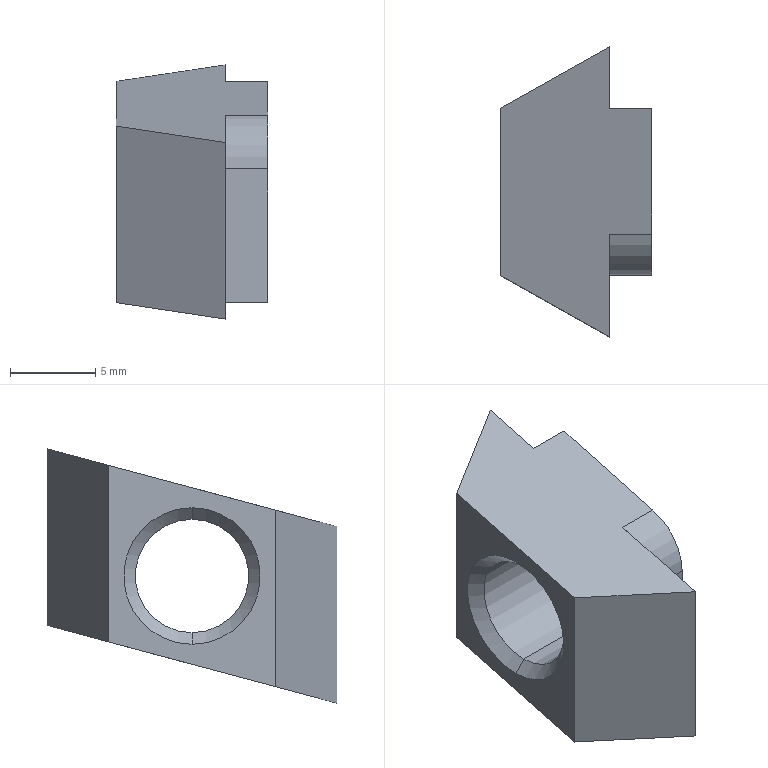Part | STEP file | 0245_014_HNTFSN8-8 | 1 solid | 18 faces | box 8.9 x 17 x 14.908 mm | volume 816.432 mm3 | plane 10 | cone 4 | cylinder 4 | commonest cylinder face diameters 6.533 x2 6.647 x2
STEP:
#1=CARTESIAN_POINT('',(0.,0.,0.));
#2=DIRECTION('',(0.,0.,1.));
#3=DIRECTION('',(1.,0.,0.));
#4=AXIS2_PLACEMENT_3D('',#1,#2,#3);
#5=CARTESIAN_POINT('',(-8.223,0.,3.323));
#6=VERTEX_POINT('',#5);
#7=CARTESIAN_POINT('',(-8.9,0.,4.));
#8=VERTEX_POINT('',#7);
#9=CARTESIAN_POINT('',(-8.9,0.,4.));
#10=DIRECTION('',(-0.7071,0.,0.7071));
#11=VECTOR('',#10,1.);
#12=LINE('',#9,#11);
#13=CARTESIAN_POINT('',(-8.9,0.,0.));
#14=DIRECTION('',(-1.,0.,0.));
#15=DIRECTION('',(0.,0.,1.));
#16=AXIS2_PLACEMENT_3D('',#13,#14,#15);
#17=CONICAL_SURFACE('',#16,4.,0.7854);
#18=CARTESIAN_POINT('',(6.283,0.));
#19=DIRECTION('',(0.,1.));
#20=VECTOR('',#19,1.);
#21=LINE('',#18,#20);
#22=(GEOMETRIC_REPRESENTATION_CONTEXT(2)PARAMETRIC_REPRESENTATION_CONTEXT()REPRESENTATION_CONTEXT('',''));
#23=DEFINITIONAL_REPRESENTATION('',(#21),#22);
#24=PCURVE('',#17,#23);
#25=CARTESIAN_POINT('',(-8.9,0.,0.));
#26=DIRECTION('',(-1.,0.,0.));
#27=DIRECTION('',(0.,0.,1.));
#28=AXIS2_PLACEMENT_3D('',#25,#26,#27);
#29=CONICAL_SURFACE('',#28,4.,0.7854);
#30=CARTESIAN_POINT('',(0.,0.));
#31=DIRECTION('',(0.,1.));
#32=VECTOR('',#31,1.);
#33=LINE('',#30,#32);
#34=(GEOMETRIC_REPRESENTATION_CONTEXT(2)PARAMETRIC_REPRESENTATION_CONTEXT()REPRESENTATION_CONTEXT('',''));
#35=DEFINITIONAL_REPRESENTATION('',(#33),#34);
#36=PCURVE('',#29,#35);
#37=SURFACE_CURVE('',#12,(#24,#36),.PCURVE_S1.);
#38=EDGE_CURVE('',#6,#8,#37,.T.);
#39=ORIENTED_EDGE('',*,*,#38,.T.);
#40=CARTESIAN_POINT('',(-8.9,0.,-4.));
#41=VERTEX_POINT('',#40);
#42=CARTESIAN_POINT('',(-8.9,0.,0.));
#43=DIRECTION('',(-1.,0.,0.));
#44=DIRECTION('',(0.,0.,1.));
#45=AXIS2_PLACEMENT_3D('',#42,#43,#44);
#46=CIRCLE('',#45,4.);
#47=CARTESIAN_POINT('',(0.,0.));
#48=DIRECTION('',(1.,0.));
#49=VECTOR('',#48,1.);
#50=LINE('',#47,#49);
#51=(GEOMETRIC_REPRESENTATION_CONTEXT(2)PARAMETRIC_REPRESENTATION_CONTEXT()REPRESENTATION_CONTEXT('',''));
#52=DEFINITIONAL_REPRESENTATION('',(#50),#51);
#53=PCURVE('',#17,#52);
#54=CARTESIAN_POINT('',(-8.9,0.,0.));
#55=DIRECTION('',(1.,0.,0.));
#56=DIRECTION('',(0.,0.,-1.));
#57=AXIS2_PLACEMENT_3D('',#54,#55,#56);
#58=PLANE('',#57);
#59=CARTESIAN_POINT('',(-4.,0.));
#60=CARTESIAN_POINT('',(-4.,6.928));
#61=CARTESIAN_POINT('',(2.,3.464));
#62=CARTESIAN_POINT('',(8.,0.));
#63=CARTESIAN_POINT('',(2.,-3.464));
#64=CARTESIAN_POINT('',(-4.,-6.928));
#65=CARTESIAN_POINT('',(-4.,0.));
#66=(BOUNDED_CURVE()B_SPLINE_CURVE(2,(#59,#60,#61,#62,#63,#64,#65),.UNSPECIFIED.,.T.,.F.)B_SPLINE_CURVE_WITH_KNOTS((1,2,2,2,2,1),(-2.094,0.,2.094,4.189,6.283,8.378),.UNSPECIFIED.)CURVE()GEOMETRIC_REPRESENTATION_ITEM()RATIONAL_B_SPLINE_CURVE((1.,0.5,1.,0.5,1.,0.5,1.))REPRESENTATION_ITEM(''));
#67=(GEOMETRIC_REPRESENTATION_CONTEXT(2)PARAMETRIC_REPRESENTATION_CONTEXT()REPRESENTATION_CONTEXT('',''));
#68=DEFINITIONAL_REPRESENTATION('',(#66),#67);
#69=PCURVE('',#58,#68);
#70=SURFACE_CURVE('',#46,(#53,#69),.PCURVE_S1.);
#71=EDGE_CURVE('',#41,#8,#70,.T.);
#72=ORIENTED_EDGE('',*,*,#71,.F.);
#73=CARTESIAN_POINT('',(-8.223,0.,-3.323));
#74=VERTEX_POINT('',#73);
#75=CARTESIAN_POINT('',(-8.9,0.,-4.));
#76=DIRECTION('',(-0.7071,0.,-0.7071));
#77=VECTOR('',#76,1.);
#78=LINE('',#75,#77);
#79=CARTESIAN_POINT('',(3.142,0.));
#80=DIRECTION('',(0.,1.));
#81=VECTOR('',#80,1.);
#82=LINE('',#79,#81);
#83=(GEOMETRIC_REPRESENTATION_CONTEXT(2)PARAMETRIC_REPRESENTATION_CONTEXT()REPRESENTATION_CONTEXT('',''));
#84=DEFINITIONAL_REPRESENTATION('',(#82),#83);
#85=PCURVE('',#17,#84);
#86=CARTESIAN_POINT('',(3.142,0.));
#87=DIRECTION('',(0.,1.));
#88=VECTOR('',#87,1.);
#89=LINE('',#86,#88);
#90=(GEOMETRIC_REPRESENTATION_CONTEXT(2)PARAMETRIC_REPRESENTATION_CONTEXT()REPRESENTATION_CONTEXT('',''));
#91=DEFINITIONAL_REPRESENTATION('',(#89),#90);
#92=PCURVE('',#29,#91);
#93=SURFACE_CURVE('',#78,(#85,#92),.PCURVE_S1.);
#94=EDGE_CURVE('',#74,#41,#93,.T.);
#95=ORIENTED_EDGE('',*,*,#94,.F.);
#96=CARTESIAN_POINT('',(-8.223,0.,0.));
#97=DIRECTION('',(-1.,0.,0.));
#98=DIRECTION('',(0.,1.,0.));
#99=AXIS2_PLACEMENT_3D('',#96,#97,#98);
#100=CIRCLE('',#99,3.323);
#101=CARTESIAN_POINT('',(1.571,-0.6765));
#102=DIRECTION('',(1.,0.));
#103=VECTOR('',#102,1.);
#104=LINE('',#101,#103);
#105=(GEOMETRIC_REPRESENTATION_CONTEXT(2)PARAMETRIC_REPRESENTATION_CONTEXT()REPRESENTATION_CONTEXT('',''));
#106=DEFINITIONAL_REPRESENTATION('',(#104),#105);
#107=PCURVE('',#17,#106);
#108=CARTESIAN_POINT('',(-4.45,0.,0.));
#109=DIRECTION('',(1.,0.,0.));
#110=DIRECTION('',(0.,0.,-1.));
#111=AXIS2_PLACEMENT_3D('',#108,#109,#110);
#112=CYLINDRICAL_SURFACE('',#111,3.324);
#113=CARTESIAN_POINT('',(7.854,-3.773));
#114=DIRECTION('',(-1.,0.));
#115=VECTOR('',#114,1.);
#116=LINE('',#113,#115);
#117=(GEOMETRIC_REPRESENTATION_CONTEXT(2)PARAMETRIC_REPRESENTATION_CONTEXT()REPRESENTATION_CONTEXT('',''));
#118=DEFINITIONAL_REPRESENTATION('',(#116),#117);
#119=PCURVE('',#112,#118);
#120=SURFACE_CURVE('',#100,(#107,#119),.PCURVE_S1.);
#121=EDGE_CURVE('',#74,#6,#120,.T.);
#122=ORIENTED_EDGE('',*,*,#121,.T.);
#123=EDGE_LOOP('',(#39,#72,#95,#122));
#124=FACE_BOUND('',#123,.F.);
#125=ADVANCED_FACE('',(#124),#17,.F.);
#126=CARTESIAN_POINT('',(-0.6765,0.,-3.324));
#127=VERTEX_POINT('',#126);
#128=CARTESIAN_POINT('',(0.,0.,-4.));
#129=VERTEX_POINT('',#128);
#130=CARTESIAN_POINT('',(0.,0.,-4.));
#131=DIRECTION('',(0.7071,0.,-0.7071));
#132=VECTOR('',#131,1.);
#133=LINE('',#130,#132);
#134=CARTESIAN_POINT('',(0.,0.,0.));
#135=DIRECTION('',(1.,0.,0.));
#136=DIRECTION('',(0.,0.,-1.));
#137=AXIS2_PLACEMENT_3D('',#134,#135,#136);
#138=CONICAL_SURFACE('',#137,4.,0.7854);
#139=CARTESIAN_POINT('',(6.283,0.));
#140=DIRECTION('',(0.,1.));
#141=VECTOR('',#140,1.);
#142=LINE('',#139,#141);
#143=(GEOMETRIC_REPRESENTATION_CONTEXT(2)PARAMETRIC_REPRESENTATION_CONTEXT()REPRESENTATION_CONTEXT('',''));
#144=DEFINITIONAL_REPRESENTATION('',(#142),#143);
#145=PCURVE('',#138,#144);
#146=CARTESIAN_POINT('',(0.,0.,0.));
#147=DIRECTION('',(1.,0.,0.));
#148=DIRECTION('',(0.,0.,-1.));
#149=AXIS2_PLACEMENT_3D('',#146,#147,#148);
#150=CONICAL_SURFACE('',#149,4.,0.7854);
#151=CARTESIAN_POINT('',(0.,0.));
#152=DIRECTION('',(0.,1.));
#153=VECTOR('',#152,1.);
#154=LINE('',#151,#153);
#155=(GEOMETRIC_REPRESENTATION_CONTEXT(2)PARAMETRIC_REPRESENTATION_CONTEXT()REPRESENTATION_CONTEXT('',''));
#156=DEFINITIONAL_REPRESENTATION('',(#154),#155);
#157=PCURVE('',#150,#156);
#158=SURFACE_CURVE('',#133,(#145,#157),.PCURVE_S1.);
#159=EDGE_CURVE('',#127,#129,#158,.T.);
#160=ORIENTED_EDGE('',*,*,#159,.T.);
#161=CARTESIAN_POINT('',(0.,0.,4.));
#162=VERTEX_POINT('',#161);
#163=CARTESIAN_POINT('',(0.,0.,0.));
#164=DIRECTION('',(-1.,0.,0.));
#165=DIRECTION('',(0.,0.,-1.));
#166=AXIS2_PLACEMENT_3D('',#163,#164,#165);
#167=CIRCLE('',#166,4.);
#168=CARTESIAN_POINT('',(6.283,0.));
#169=DIRECTION('',(-1.,0.));
#170=VECTOR('',#169,1.);
#171=LINE('',#168,#170);
#172=(GEOMETRIC_REPRESENTATION_CONTEXT(2)PARAMETRIC_REPRESENTATION_CONTEXT()REPRESENTATION_CONTEXT('',''));
#173=DEFINITIONAL_REPRESENTATION('',(#171),#172);
#174=PCURVE('',#138,#173);
#175=CARTESIAN_POINT('',(0.,0.,0.));
#176=DIRECTION('',(1.,0.,0.));
#177=DIRECTION('',(0.,0.,-1.));
#178=AXIS2_PLACEMENT_3D('',#175,#176,#177);
#179=PLANE('',#178);
#180=CARTESIAN_POINT('',(4.,0.));
#181=CARTESIAN_POINT('',(4.,-6.928));
#182=CARTESIAN_POINT('',(-2.,-3.464));
#183=CARTESIAN_POINT('',(-8.,0.));
#184=CARTESIAN_POINT('',(-2.,3.464));
#185=CARTESIAN_POINT('',(4.,6.928));
#186=CARTESIAN_POINT('',(4.,0.));
#187=(BOUNDED_CURVE()B_SPLINE_CURVE(2,(#180,#181,#182,#183,#184,#185,#186),.UNSPECIFIED.,.T.,.F.)B_SPLINE_CURVE_WITH_KNOTS((1,2,2,2,2,1),(-2.094,0.,2.094,4.189,6.283,8.378),.UNSPECIFIED.)CURVE()GEOMETRIC_REPRESENTATION_ITEM()RATIONAL_B_SPLINE_CURVE((1.,0.5,1.,0.5,1.,0.5,1.))REPRESENTATION_ITEM(''));
#188=(GEOMETRIC_REPRESENTATION_CONTEXT(2)PARAMETRIC_REPRESENTATION_CONTEXT()REPRESENTATION_CONTEXT('',''));
#189=DEFINITIONAL_REPRESENTATION('',(#187),#188);
#190=PCURVE('',#179,#189);
#191=SURFACE_CURVE('',#167,(#174,#190),.PCURVE_S1.);
#192=EDGE_CURVE('',#129,#162,#191,.T.);
#193=ORIENTED_EDGE('',*,*,#192,.T.);
#194=CARTESIAN_POINT('',(-0.6765,0.,3.324));
#195=VERTEX_POINT('',#194);
#196=CARTESIAN_POINT('',(0.,0.,4.));
#197=DIRECTION('',(0.7071,0.,0.7071));
#198=VECTOR('',#197,1.);
#199=LINE('',#196,#198);
#200=CARTESIAN_POINT('',(3.142,0.));
#201=DIRECTION('',(0.,1.));
#202=VECTOR('',#201,1.);
#203=LINE('',#200,#202);
#204=(GEOMETRIC_REPRESENTATION_CONTEXT(2)PARAMETRIC_REPRESENTATION_CONTEXT()REPRESENTATION_CONTEXT('',''));
#205=DEFINITIONAL_REPRESENTATION('',(#203),#204);
#206=PCURVE('',#138,#205);
#207=CARTESIAN_POINT('',(3.142,0.));
#208=DIRECTION('',(0.,1.));
#209=VECTOR('',#208,1.);
#210=LINE('',#207,#209);
#211=(GEOMETRIC_REPRESENTATION_CONTEXT(2)PARAMETRIC_REPRESENTATION_CONTEXT()REPRESENTATION_CONTEXT('',''));
#212=DEFINITIONAL_REPRESENTATION('',(#210),#211);
#213=PCURVE('',#150,#212);
#214=SURFACE_CURVE('',#199,(#206,#213),.PCURVE_S1.);
#215=EDGE_CURVE('',#195,#162,#214,.T.);
#216=ORIENTED_EDGE('',*,*,#215,.F.);
#217=CARTESIAN_POINT('',(-0.6765,0.,0.));
#218=DIRECTION('',(1.,0.,0.));
#219=DIRECTION('',(0.,1.,0.));
#220=AXIS2_PLACEMENT_3D('',#217,#218,#219);
#221=CIRCLE('',#220,3.324);
#222=CARTESIAN_POINT('',(1.571,-0.6765));
#223=DIRECTION('',(1.,0.));
#224=VECTOR('',#223,1.);
#225=LINE('',#222,#224);
#226=(GEOMETRIC_REPRESENTATION_CONTEXT(2)PARAMETRIC_REPRESENTATION_CONTEXT()REPRESENTATION_CONTEXT('',''));
#227=DEFINITIONAL_REPRESENTATION('',(#225),#226);
#228=PCURVE('',#138,#227);
#229=CARTESIAN_POINT('',(1.571,3.774));
#230=DIRECTION('',(1.,0.));
#231=VECTOR('',#230,1.);
#232=LINE('',#229,#231);
#233=(GEOMETRIC_REPRESENTATION_CONTEXT(2)PARAMETRIC_REPRESENTATION_CONTEXT()REPRESENTATION_CONTEXT('',''));
#234=DEFINITIONAL_REPRESENTATION('',(#232),#233);
#235=PCURVE('',#112,#234);
#236=SURFACE_CURVE('',#221,(#228,#235),.PCURVE_S1.);
#237=EDGE_CURVE('',#195,#127,#236,.T.);
#238=ORIENTED_EDGE('',*,*,#237,.T.);
#239=EDGE_LOOP('',(#160,#193,#216,#238));
#240=FACE_BOUND('',#239,.F.);
#241=ADVANCED_FACE('',(#240),#138,.F.);
#242=CARTESIAN_POINT('',(-4.45,0.,-3.324));
#243=DIRECTION('',(1.,0.,0.));
#244=VECTOR('',#243,1.);
#245=LINE('',#242,#244);
#246=CARTESIAN_POINT('',(6.283,0.));
#247=DIRECTION('',(0.,1.));
#248=VECTOR('',#247,1.);
#249=LINE('',#246,#248);
#250=(GEOMETRIC_REPRESENTATION_CONTEXT(2)PARAMETRIC_REPRESENTATION_CONTEXT()REPRESENTATION_CONTEXT('',''));
#251=DEFINITIONAL_REPRESENTATION('',(#249),#250);
#252=PCURVE('',#112,#251);
#253=CARTESIAN_POINT('',(-4.45,0.,0.));
#254=DIRECTION('',(1.,0.,0.));
#255=DIRECTION('',(0.,0.,-1.));
#256=AXIS2_PLACEMENT_3D('',#253,#254,#255);
#257=CYLINDRICAL_SURFACE('',#256,3.324);
#258=CARTESIAN_POINT('',(0.,0.));
#259=DIRECTION('',(0.,1.));
#260=VECTOR('',#259,1.);
#261=LINE('',#258,#260);
#262=(GEOMETRIC_REPRESENTATION_CONTEXT(2)PARAMETRIC_REPRESENTATION_CONTEXT()REPRESENTATION_CONTEXT('',''));
#263=DEFINITIONAL_REPRESENTATION('',(#261),#262);
#264=PCURVE('',#257,#263);
#265=SURFACE_CURVE('',#245,(#252,#264),.PCURVE_S1.);
#266=EDGE_CURVE('',#74,#127,#265,.T.);
#267=ORIENTED_EDGE('',*,*,#266,.T.);
#268=ORIENTED_EDGE('',*,*,#237,.F.);
#269=CARTESIAN_POINT('',(-4.45,0.,3.324));
#270=DIRECTION('',(1.,0.,0.));
#271=VECTOR('',#270,1.);
#272=LINE('',#269,#271);
#273=CARTESIAN_POINT('',(3.142,0.));
#274=DIRECTION('',(0.,1.));
#275=VECTOR('',#274,1.);
#276=LINE('',#273,#275);
#277=(GEOMETRIC_REPRESENTATION_CONTEXT(2)PARAMETRIC_REPRESENTATION_CONTEXT()REPRESENTATION_CONTEXT('',''));
#278=DEFINITIONAL_REPRESENTATION('',(#276),#277);
#279=PCURVE('',#112,#278);
#280=CARTESIAN_POINT('',(3.142,0.));
#281=DIRECTION('',(0.,1.));
#282=VECTOR('',#281,1.);
#283=LINE('',#280,#282);
#284=(GEOMETRIC_REPRESENTATION_CONTEXT(2)PARAMETRIC_REPRESENTATION_CONTEXT()REPRESENTATION_CONTEXT('',''));
#285=DEFINITIONAL_REPRESENTATION('',(#283),#284);
#286=PCURVE('',#257,#285);
#287=SURFACE_CURVE('',#272,(#279,#286),.PCURVE_S1.);
#288=EDGE_CURVE('',#6,#195,#287,.T.);
#289=ORIENTED_EDGE('',*,*,#288,.F.);
#290=ORIENTED_EDGE('',*,*,#121,.F.);
#291=EDGE_LOOP('',(#267,#268,#289,#290));
#292=FACE_BOUND('',#291,.F.);
#293=ADVANCED_FACE('',(#292),#112,.F.);
#294=CARTESIAN_POINT('',(-8.9,-4.9,3.863));
#295=VERTEX_POINT('',#294);
#296=CARTESIAN_POINT('',(-2.5,-8.5,2.899));
#297=VERTEX_POINT('',#296);
#298=CARTESIAN_POINT('',(-8.9,-4.9,3.863));
#299=DIRECTION('',(0.8642,-0.4861,-0.1302));
#300=VECTOR('',#299,1.);
#301=LINE('',#298,#300);
#302=CARTESIAN_POINT('',(0.,8.5,7.454));
#303=DIRECTION('',(0.,-0.2588,0.9659));
#304=DIRECTION('',(0.,-0.9659,-0.2588));
#305=AXIS2_PLACEMENT_3D('',#302,#303,#304);
#306=PLANE('',#305);
#307=CARTESIAN_POINT('',(13.873,-8.9));
#308=DIRECTION('',(0.5032,0.8642));
#309=VECTOR('',#308,1.);
#310=LINE('',#307,#309);
#311=(GEOMETRIC_REPRESENTATION_CONTEXT(2)PARAMETRIC_REPRESENTATION_CONTEXT()REPRESENTATION_CONTEXT('',''));
#312=DEFINITIONAL_REPRESENTATION('',(#310),#311);
#313=PCURVE('',#306,#312);
#314=CARTESIAN_POINT('',(-2.5,-8.5,20.));
#315=DIRECTION('',(0.4903,0.8716,0.));
#316=DIRECTION('',(-0.8716,0.4903,0.));
#317=AXIS2_PLACEMENT_3D('',#314,#315,#316);
#318=PLANE('',#317);
#319=CARTESIAN_POINT('',(7.343,-16.137));
#320=DIRECTION('',(-0.9915,-0.1302));
#321=VECTOR('',#320,1.);
#322=LINE('',#319,#321);
#323=(GEOMETRIC_REPRESENTATION_CONTEXT(2)PARAMETRIC_REPRESENTATION_CONTEXT()REPRESENTATION_CONTEXT('',''));
#324=DEFINITIONAL_REPRESENTATION('',(#322),#323);
#325=PCURVE('',#318,#324);
#326=SURFACE_CURVE('',#301,(#313,#325),.PCURVE_S1.);
#327=EDGE_CURVE('',#295,#297,#326,.T.);
#328=ORIENTED_EDGE('',*,*,#327,.T.);
#329=CARTESIAN_POINT('',(-2.5,-2.479,4.512));
#330=VERTEX_POINT('',#329);
#331=CARTESIAN_POINT('',(-2.5,8.5,7.454));
#332=DIRECTION('',(0.,0.9659,0.2588));
#333=VECTOR('',#332,1.);
#334=LINE('',#331,#333);
#335=CARTESIAN_POINT('',(0.,-2.5));
#336=DIRECTION('',(-1.,0.));
#337=VECTOR('',#336,1.);
#338=LINE('',#335,#337);
#339=(GEOMETRIC_REPRESENTATION_CONTEXT(2)PARAMETRIC_REPRESENTATION_CONTEXT()REPRESENTATION_CONTEXT('',''));
#340=DEFINITIONAL_REPRESENTATION('',(#338),#339);
#341=PCURVE('',#306,#340);
#342=CARTESIAN_POINT('',(-2.5,-4.9,20.));
#343=DIRECTION('',(-1.,0.,0.));
#344=DIRECTION('',(0.,0.,1.));
#345=AXIS2_PLACEMENT_3D('',#342,#343,#344);
#346=PLANE('',#345);
#347=CARTESIAN_POINT('',(-12.546,13.4));
#348=DIRECTION('',(0.2588,0.9659));
#349=VECTOR('',#348,1.);
#350=LINE('',#347,#349);
#351=(GEOMETRIC_REPRESENTATION_CONTEXT(2)PARAMETRIC_REPRESENTATION_CONTEXT()REPRESENTATION_CONTEXT('',''));
#352=DEFINITIONAL_REPRESENTATION('',(#350),#351);
#353=PCURVE('',#346,#352);
#354=SURFACE_CURVE('',#334,(#341,#353),.PCURVE_S1.);
#355=EDGE_CURVE('',#297,#330,#354,.T.);
#356=ORIENTED_EDGE('',*,*,#355,.T.);
#357=CARTESIAN_POINT('',(0.,-2.479,4.512));
#358=VERTEX_POINT('',#357);
#359=CARTESIAN_POINT('',(0.,-2.479,4.512));
#360=DIRECTION('',(1.,0.,0.));
#361=VECTOR('',#360,1.);
#362=LINE('',#359,#361);
#363=CARTESIAN_POINT('',(11.366,0.));
#364=DIRECTION('',(0.,1.));
#365=VECTOR('',#364,1.);
#366=LINE('',#363,#365);
#367=(GEOMETRIC_REPRESENTATION_CONTEXT(2)PARAMETRIC_REPRESENTATION_CONTEXT()REPRESENTATION_CONTEXT('',''));
#368=DEFINITIONAL_REPRESENTATION('',(#366),#367);
#369=PCURVE('',#306,#368);
#370=CARTESIAN_POINT('',(-2.5,-1.633,1.357));
#371=DIRECTION('',(-1.,0.,0.));
#372=DIRECTION('',(0.,0.,1.));
#373=AXIS2_PLACEMENT_3D('',#370,#371,#372);
#374=CYLINDRICAL_SURFACE('',#373,3.267);
#375=CARTESIAN_POINT('',(6.021,-2.5));
#376=DIRECTION('',(0.,-1.));
#377=VECTOR('',#376,1.);
#378=LINE('',#375,#377);
#379=(GEOMETRIC_REPRESENTATION_CONTEXT(2)PARAMETRIC_REPRESENTATION_CONTEXT()REPRESENTATION_CONTEXT('',''));
#380=DEFINITIONAL_REPRESENTATION('',(#378),#379);
#381=PCURVE('',#374,#380);
#382=SURFACE_CURVE('',#362,(#369,#381),.PCURVE_S1.);
#383=EDGE_CURVE('',#330,#358,#382,.T.);
#384=ORIENTED_EDGE('',*,*,#383,.T.);
#385=CARTESIAN_POINT('',(0.,4.9,6.489));
#386=VERTEX_POINT('',#385);
#387=CARTESIAN_POINT('',(0.,8.5,7.454));
#388=DIRECTION('',(0.,0.9659,0.2588));
#389=VECTOR('',#388,1.);
#390=LINE('',#387,#389);
#391=CARTESIAN_POINT('',(0.,0.));
#392=DIRECTION('',(-1.,0.));
#393=VECTOR('',#392,1.);
#394=LINE('',#391,#393);
#395=(GEOMETRIC_REPRESENTATION_CONTEXT(2)PARAMETRIC_REPRESENTATION_CONTEXT()REPRESENTATION_CONTEXT('',''));
#396=DEFINITIONAL_REPRESENTATION('',(#394),#395);
#397=PCURVE('',#306,#396);
#398=CARTESIAN_POINT('',(-7.454,8.5));
#399=DIRECTION('',(-0.2588,0.9659));
#400=VECTOR('',#399,1.);
#401=LINE('',#398,#400);
#402=(GEOMETRIC_REPRESENTATION_CONTEXT(2)PARAMETRIC_REPRESENTATION_CONTEXT()REPRESENTATION_CONTEXT('',''));
#403=DEFINITIONAL_REPRESENTATION('',(#401),#402);
#404=PCURVE('',#179,#403);
#405=SURFACE_CURVE('',#390,(#397,#404),.PCURVE_S1.);
#406=EDGE_CURVE('',#358,#386,#405,.T.);
#407=ORIENTED_EDGE('',*,*,#406,.T.);
#408=CARTESIAN_POINT('',(-2.5,4.9,6.489));
#409=VERTEX_POINT('',#408);
#410=CARTESIAN_POINT('',(0.,4.9,6.489));
#411=DIRECTION('',(-1.,0.,0.));
#412=VECTOR('',#411,1.);
#413=LINE('',#410,#412);
#414=CARTESIAN_POINT('',(3.727,0.));
#415=DIRECTION('',(0.,-1.));
#416=VECTOR('',#415,1.);
#417=LINE('',#414,#416);
#418=(GEOMETRIC_REPRESENTATION_CONTEXT(2)PARAMETRIC_REPRESENTATION_CONTEXT()REPRESENTATION_CONTEXT('',''));
#419=DEFINITIONAL_REPRESENTATION('',(#417),#418);
#420=PCURVE('',#306,#419);
#421=CARTESIAN_POINT('',(-2.5,4.9,20.));
#422=DIRECTION('',(0.,-1.,0.));
#423=DIRECTION('',(1.,0.,0.));
#424=AXIS2_PLACEMENT_3D('',#421,#422,#423);
#425=PLANE('',#424);
#426=CARTESIAN_POINT('',(2.5,-13.511));
#427=DIRECTION('',(-1.,0.));
#428=VECTOR('',#427,1.);
#429=LINE('',#426,#428);
#430=(GEOMETRIC_REPRESENTATION_CONTEXT(2)PARAMETRIC_REPRESENTATION_CONTEXT()REPRESENTATION_CONTEXT('',''));
#431=DEFINITIONAL_REPRESENTATION('',(#429),#430);
#432=PCURVE('',#425,#431);
#433=SURFACE_CURVE('',#413,(#420,#432),.PCURVE_S1.);
#434=EDGE_CURVE('',#386,#409,#433,.T.);
#435=ORIENTED_EDGE('',*,*,#434,.T.);
#436=CARTESIAN_POINT('',(-2.5,8.5,7.454));
#437=VERTEX_POINT('',#436);
#438=CARTESIAN_POINT('',(-2.5,8.5,7.454));
#439=DIRECTION('',(0.,0.9659,0.2588));
#440=VECTOR('',#439,1.);
#441=LINE('',#438,#440);
#442=CARTESIAN_POINT('',(0.,-2.5));
#443=DIRECTION('',(-1.,0.));
#444=VECTOR('',#443,1.);
#445=LINE('',#442,#444);
#446=(GEOMETRIC_REPRESENTATION_CONTEXT(2)PARAMETRIC_REPRESENTATION_CONTEXT()REPRESENTATION_CONTEXT('',''));
#447=DEFINITIONAL_REPRESENTATION('',(#445),#446);
#448=PCURVE('',#306,#447);
#449=CARTESIAN_POINT('',(-2.5,8.5,20.));
#450=DIRECTION('',(-1.,0.,0.));
#451=DIRECTION('',(0.,0.,1.));
#452=AXIS2_PLACEMENT_3D('',#449,#450,#451);
#453=PLANE('',#452);
#454=CARTESIAN_POINT('',(-12.546,0.));
#455=DIRECTION('',(0.2588,0.9659));
#456=VECTOR('',#455,1.);
#457=LINE('',#454,#456);
#458=(GEOMETRIC_REPRESENTATION_CONTEXT(2)PARAMETRIC_REPRESENTATION_CONTEXT()REPRESENTATION_CONTEXT('',''));
#459=DEFINITIONAL_REPRESENTATION('',(#457),#458);
#460=PCURVE('',#453,#459);
#461=SURFACE_CURVE('',#441,(#448,#460),.PCURVE_S1.);
#462=EDGE_CURVE('',#409,#437,#461,.T.);
#463=ORIENTED_EDGE('',*,*,#462,.T.);
#464=CARTESIAN_POINT('',(-8.9,4.9,6.489));
#465=VERTEX_POINT('',#464);
#466=CARTESIAN_POINT('',(-2.5,8.5,7.454));
#467=DIRECTION('',(-0.8642,-0.4861,-0.1302));
#468=VECTOR('',#467,1.);
#469=LINE('',#466,#468);
#470=CARTESIAN_POINT('',(0.,-2.5));
#471=DIRECTION('',(0.5032,-0.8642));
#472=VECTOR('',#471,1.);
#473=LINE('',#470,#472);
#474=(GEOMETRIC_REPRESENTATION_CONTEXT(2)PARAMETRIC_REPRESENTATION_CONTEXT()REPRESENTATION_CONTEXT('',''));
#475=DEFINITIONAL_REPRESENTATION('',(#473),#474);
#476=PCURVE('',#306,#475);
#477=CARTESIAN_POINT('',(-8.9,4.9,20.));
#478=DIRECTION('',(0.4903,-0.8716,0.));
#479=DIRECTION('',(0.8716,0.4903,0.));
#480=AXIS2_PLACEMENT_3D('',#477,#478,#479);
#481=PLANE('',#480);
#482=CARTESIAN_POINT('',(7.343,-12.546));
#483=DIRECTION('',(-0.9915,-0.1302));
#484=VECTOR('',#483,1.);
#485=LINE('',#482,#484);
#486=(GEOMETRIC_REPRESENTATION_CONTEXT(2)PARAMETRIC_REPRESENTATION_CONTEXT()REPRESENTATION_CONTEXT('',''));
#487=DEFINITIONAL_REPRESENTATION('',(#485),#486);
#488=PCURVE('',#481,#487);
#489=SURFACE_CURVE('',#469,(#476,#488),.PCURVE_S1.);
#490=EDGE_CURVE('',#437,#465,#489,.T.);
#491=ORIENTED_EDGE('',*,*,#490,.T.);
#492=CARTESIAN_POINT('',(-8.9,8.5,7.454));
#493=DIRECTION('',(0.,-0.9659,-0.2588));
#494=VECTOR('',#493,1.);
#495=LINE('',#492,#494);
#496=CARTESIAN_POINT('',(0.,-8.9));
#497=DIRECTION('',(1.,0.));
#498=VECTOR('',#497,1.);
#499=LINE('',#496,#498);
#500=(GEOMETRIC_REPRESENTATION_CONTEXT(2)PARAMETRIC_REPRESENTATION_CONTEXT()REPRESENTATION_CONTEXT('',''));
#501=DEFINITIONAL_REPRESENTATION('',(#499),#500);
#502=PCURVE('',#306,#501);
#503=CARTESIAN_POINT('',(-7.454,8.5));
#504=DIRECTION('',(0.2588,-0.9659));
#505=VECTOR('',#504,1.);
#506=LINE('',#503,#505);
#507=(GEOMETRIC_REPRESENTATION_CONTEXT(2)PARAMETRIC_REPRESENTATION_CONTEXT()REPRESENTATION_CONTEXT('',''));
#508=DEFINITIONAL_REPRESENTATION('',(#506),#507);
#509=PCURVE('',#58,#508);
#510=SURFACE_CURVE('',#495,(#502,#509),.PCURVE_S1.);
#511=EDGE_CURVE('',#465,#295,#510,.T.);
#512=ORIENTED_EDGE('',*,*,#511,.T.);
#513=EDGE_LOOP('',(#328,#356,#384,#407,#435,#463,#491,#512));
#514=FACE_BOUND('',#513,.T.);
#515=ADVANCED_FACE('',(#514),#306,.T.);
#516=CARTESIAN_POINT('',(-2.5,-8.5,-7.454));
#517=VERTEX_POINT('',#516);
#518=CARTESIAN_POINT('',(-2.5,-8.5,20.));
#519=DIRECTION('',(0.,0.,1.));
#520=VECTOR('',#519,1.);
#521=LINE('',#518,#520);
#522=CARTESIAN_POINT('',(0.,-3.6));
#523=DIRECTION('',(1.,0.));
#524=VECTOR('',#523,1.);
#525=LINE('',#522,#524);
#526=(GEOMETRIC_REPRESENTATION_CONTEXT(2)PARAMETRIC_REPRESENTATION_CONTEXT()REPRESENTATION_CONTEXT('',''));
#527=DEFINITIONAL_REPRESENTATION('',(#525),#526);
#528=PCURVE('',#346,#527);
#529=CARTESIAN_POINT('',(0.,0.));
#530=DIRECTION('',(0.,1.));
#531=VECTOR('',#530,1.);
#532=LINE('',#529,#531);
#533=(GEOMETRIC_REPRESENTATION_CONTEXT(2)PARAMETRIC_REPRESENTATION_CONTEXT()REPRESENTATION_CONTEXT('',''));
#534=DEFINITIONAL_REPRESENTATION('',(#532),#533);
#535=PCURVE('',#318,#534);
#536=SURFACE_CURVE('',#521,(#528,#535),.PCURVE_S1.);
#537=EDGE_CURVE('',#517,#297,#536,.T.);
#538=ORIENTED_EDGE('',*,*,#537,.F.);
#539=CARTESIAN_POINT('',(-2.5,-4.9,-6.489));
#540=VERTEX_POINT('',#539);
#541=CARTESIAN_POINT('',(-2.5,-4.9,-6.489));
#542=DIRECTION('',(0.,-0.9659,-0.2588));
#543=VECTOR('',#542,1.);
#544=LINE('',#541,#543);
#545=CARTESIAN_POINT('',(-26.489,0.));
#546=DIRECTION('',(-0.2588,-0.9659));
#547=VECTOR('',#546,1.);
#548=LINE('',#545,#547);
#549=(GEOMETRIC_REPRESENTATION_CONTEXT(2)PARAMETRIC_REPRESENTATION_CONTEXT()REPRESENTATION_CONTEXT('',''));
#550=DEFINITIONAL_REPRESENTATION('',(#548),#549);
#551=PCURVE('',#346,#550);
#552=CARTESIAN_POINT('',(0.,-8.5,-7.454));
#553=DIRECTION('',(0.,0.2588,-0.9659));
#554=DIRECTION('',(0.,0.9659,0.2588));
#555=AXIS2_PLACEMENT_3D('',#552,#553,#554);
#556=PLANE('',#555);
#557=CARTESIAN_POINT('',(3.727,-2.5));
#558=DIRECTION('',(-1.,0.));
#559=VECTOR('',#558,1.);
#560=LINE('',#557,#559);
#561=(GEOMETRIC_REPRESENTATION_CONTEXT(2)PARAMETRIC_REPRESENTATION_CONTEXT()REPRESENTATION_CONTEXT('',''));
#562=DEFINITIONAL_REPRESENTATION('',(#560),#561);
#563=PCURVE('',#556,#562);
#564=SURFACE_CURVE('',#544,(#551,#563),.PCURVE_S1.);
#565=EDGE_CURVE('',#540,#517,#564,.T.);
#566=ORIENTED_EDGE('',*,*,#565,.F.);
#567=CARTESIAN_POINT('',(-2.5,-4.9,1.357));
#568=VERTEX_POINT('',#567);
#569=CARTESIAN_POINT('',(-2.5,-4.9,20.));
#570=DIRECTION('',(0.,0.,-1.));
#571=VECTOR('',#570,1.);
#572=LINE('',#569,#571);
#573=CARTESIAN_POINT('',(0.,0.));
#574=DIRECTION('',(-1.,0.));
#575=VECTOR('',#574,1.);
#576=LINE('',#573,#575);
#577=(GEOMETRIC_REPRESENTATION_CONTEXT(2)PARAMETRIC_REPRESENTATION_CONTEXT()REPRESENTATION_CONTEXT('',''));
#578=DEFINITIONAL_REPRESENTATION('',(#576),#577);
#579=PCURVE('',#346,#578);
#580=CARTESIAN_POINT('',(0.,-4.9,20.));
#581=DIRECTION('',(0.,1.,0.));
#582=DIRECTION('',(-1.,0.,0.));
#583=AXIS2_PLACEMENT_3D('',#580,#581,#582);
#584=PLANE('',#583);
#585=CARTESIAN_POINT('',(2.5,0.));
#586=DIRECTION('',(0.,-1.));
#587=VECTOR('',#586,1.);
#588=LINE('',#585,#587);
#589=(GEOMETRIC_REPRESENTATION_CONTEXT(2)PARAMETRIC_REPRESENTATION_CONTEXT()REPRESENTATION_CONTEXT('',''));
#590=DEFINITIONAL_REPRESENTATION('',(#588),#589);
#591=PCURVE('',#584,#590);
#592=SURFACE_CURVE('',#572,(#579,#591),.PCURVE_S1.);
#593=EDGE_CURVE('',#568,#540,#592,.T.);
#594=ORIENTED_EDGE('',*,*,#593,.F.);
#595=CARTESIAN_POINT('',(-2.5,-1.633,1.357));
#596=DIRECTION('',(1.,0.,0.));
#597=DIRECTION('',(0.,0.,1.));
#598=AXIS2_PLACEMENT_3D('',#595,#596,#597);
#599=CIRCLE('',#598,3.267);
#600=CARTESIAN_POINT('',(-15.377,3.267));
#601=CARTESIAN_POINT('',(-15.377,-2.391));
#602=CARTESIAN_POINT('',(-20.277,0.4377));
#603=CARTESIAN_POINT('',(-25.177,3.267));
#604=CARTESIAN_POINT('',(-20.277,6.096));
#605=CARTESIAN_POINT('',(-15.377,8.925));
#606=CARTESIAN_POINT('',(-15.377,3.267));
#607=(BOUNDED_CURVE()B_SPLINE_CURVE(2,(#600,#601,#602,#603,#604,#605,#606),.UNSPECIFIED.,.T.,.F.)B_SPLINE_CURVE_WITH_KNOTS((1,2,2,2,2,1),(-2.094,0.,2.094,4.189,6.283,8.378),.UNSPECIFIED.)CURVE()GEOMETRIC_REPRESENTATION_ITEM()RATIONAL_B_SPLINE_CURVE((1.,0.5,1.,0.5,1.,0.5,1.))REPRESENTATION_ITEM(''));
#608=(GEOMETRIC_REPRESENTATION_CONTEXT(2)PARAMETRIC_REPRESENTATION_CONTEXT()REPRESENTATION_CONTEXT('',''));
#609=DEFINITIONAL_REPRESENTATION('',(#607),#608);
#610=PCURVE('',#346,#609);
#611=CARTESIAN_POINT('',(6.283,0.));
#612=DIRECTION('',(-1.,0.));
#613=VECTOR('',#612,1.);
#614=LINE('',#611,#613);
#615=(GEOMETRIC_REPRESENTATION_CONTEXT(2)PARAMETRIC_REPRESENTATION_CONTEXT()REPRESENTATION_CONTEXT('',''));
#616=DEFINITIONAL_REPRESENTATION('',(#614),#615);
#617=PCURVE('',#374,#616);
#618=SURFACE_CURVE('',#599,(#610,#617),.PCURVE_S1.);
#619=EDGE_CURVE('',#330,#568,#618,.T.);
#620=ORIENTED_EDGE('',*,*,#619,.F.);
#621=ORIENTED_EDGE('',*,*,#355,.F.);
#622=EDGE_LOOP('',(#538,#566,#594,#620,#621));
#623=FACE_BOUND('',#622,.T.);
#624=ADVANCED_FACE('',(#623),#346,.F.);
#625=ORIENTED_EDGE('',*,*,#537,.T.);
#626=ORIENTED_EDGE('',*,*,#327,.F.);
#627=CARTESIAN_POINT('',(-8.9,-4.9,-6.489));
#628=VERTEX_POINT('',#627);
#629=CARTESIAN_POINT('',(-8.9,-4.9,20.));
#630=DIRECTION('',(0.,0.,1.));
#631=VECTOR('',#630,1.);
#632=LINE('',#629,#631);
#633=CARTESIAN_POINT('',(7.343,0.));
#634=DIRECTION('',(0.,1.));
#635=VECTOR('',#634,1.);
#636=LINE('',#633,#635);
#637=(GEOMETRIC_REPRESENTATION_CONTEXT(2)PARAMETRIC_REPRESENTATION_CONTEXT()REPRESENTATION_CONTEXT('',''));
#638=DEFINITIONAL_REPRESENTATION('',(#636),#637);
#639=PCURVE('',#318,#638);
#640=CARTESIAN_POINT('',(-20.,-4.9));
#641=DIRECTION('',(-1.,0.));
#642=VECTOR('',#641,1.);
#643=LINE('',#640,#642);
#644=(GEOMETRIC_REPRESENTATION_CONTEXT(2)PARAMETRIC_REPRESENTATION_CONTEXT()REPRESENTATION_CONTEXT('',''));
#645=DEFINITIONAL_REPRESENTATION('',(#643),#644);
#646=PCURVE('',#58,#645);
#647=SURFACE_CURVE('',#632,(#639,#646),.PCURVE_S1.);
#648=EDGE_CURVE('',#628,#295,#647,.T.);
#649=ORIENTED_EDGE('',*,*,#648,.F.);
#650=CARTESIAN_POINT('',(-2.5,-8.5,-7.454));
#651=DIRECTION('',(-0.8642,0.4861,0.1302));
#652=VECTOR('',#651,1.);
#653=LINE('',#650,#652);
#654=CARTESIAN_POINT('',(0.,-27.454));
#655=DIRECTION('',(0.9915,0.1302));
#656=VECTOR('',#655,1.);
#657=LINE('',#654,#656);
#658=(GEOMETRIC_REPRESENTATION_CONTEXT(2)PARAMETRIC_REPRESENTATION_CONTEXT()REPRESENTATION_CONTEXT('',''));
#659=DEFINITIONAL_REPRESENTATION('',(#657),#658);
#660=PCURVE('',#318,#659);
#661=CARTESIAN_POINT('',(0.,-2.5));
#662=DIRECTION('',(0.5032,-0.8642));
#663=VECTOR('',#662,1.);
#664=LINE('',#661,#663);
#665=(GEOMETRIC_REPRESENTATION_CONTEXT(2)PARAMETRIC_REPRESENTATION_CONTEXT()REPRESENTATION_CONTEXT('',''));
#666=DEFINITIONAL_REPRESENTATION('',(#664),#665);
#667=PCURVE('',#556,#666);
#668=SURFACE_CURVE('',#653,(#660,#667),.PCURVE_S1.);
#669=EDGE_CURVE('',#517,#628,#668,.T.);
#670=ORIENTED_EDGE('',*,*,#669,.F.);
#671=EDGE_LOOP('',(#625,#626,#649,#670));
#672=FACE_BOUND('',#671,.T.);
#673=ADVANCED_FACE('',(#672),#318,.F.);
#674=CARTESIAN_POINT('',(-8.9,4.9,-3.863));
#675=VERTEX_POINT('',#674);
#676=CARTESIAN_POINT('',(-8.9,-4.9,-6.489));
#677=DIRECTION('',(0.,0.9659,0.2588));
#678=VECTOR('',#677,1.);
#679=LINE('',#676,#678);
#680=CARTESIAN_POINT('',(6.489,-4.9));
#681=DIRECTION('',(-0.2588,0.9659));
#682=VECTOR('',#681,1.);
#683=LINE('',#680,#682);
#684=(GEOMETRIC_REPRESENTATION_CONTEXT(2)PARAMETRIC_REPRESENTATION_CONTEXT()REPRESENTATION_CONTEXT('',''));
#685=DEFINITIONAL_REPRESENTATION('',(#683),#684);
#686=PCURVE('',#58,#685);
#687=CARTESIAN_POINT('',(3.727,-8.9));
#688=DIRECTION('',(1.,0.));
#689=VECTOR('',#688,1.);
#690=LINE('',#687,#689);
#691=(GEOMETRIC_REPRESENTATION_CONTEXT(2)PARAMETRIC_REPRESENTATION_CONTEXT()REPRESENTATION_CONTEXT('',''));
#692=DEFINITIONAL_REPRESENTATION('',(#690),#691);
#693=PCURVE('',#556,#692);
#694=SURFACE_CURVE('',#679,(#686,#693),.PCURVE_S1.);
#695=EDGE_CURVE('',#628,#675,#694,.T.);
#696=ORIENTED_EDGE('',*,*,#695,.F.);
#697=ORIENTED_EDGE('',*,*,#648,.T.);
#698=ORIENTED_EDGE('',*,*,#511,.F.);
#699=CARTESIAN_POINT('',(-8.9,4.9,0.));
#700=DIRECTION('',(0.,0.,1.));
#701=VECTOR('',#700,1.);
#702=LINE('',#699,#701);
#703=CARTESIAN_POINT('',(0.,4.9));
#704=DIRECTION('',(-1.,0.));
#705=VECTOR('',#704,1.);
#706=LINE('',#703,#705);
#707=(GEOMETRIC_REPRESENTATION_CONTEXT(2)PARAMETRIC_REPRESENTATION_CONTEXT()REPRESENTATION_CONTEXT('',''));
#708=DEFINITIONAL_REPRESENTATION('',(#706),#707);
#709=PCURVE('',#58,#708);
#710=CARTESIAN_POINT('',(0.,-20.));
#711=DIRECTION('',(0.,1.));
#712=VECTOR('',#711,1.);
#713=LINE('',#710,#712);
#714=(GEOMETRIC_REPRESENTATION_CONTEXT(2)PARAMETRIC_REPRESENTATION_CONTEXT()REPRESENTATION_CONTEXT('',''));
#715=DEFINITIONAL_REPRESENTATION('',(#713),#714);
#716=PCURVE('',#481,#715);
#717=SURFACE_CURVE('',#702,(#709,#716),.PCURVE_S1.);
#718=EDGE_CURVE('',#675,#465,#717,.T.);
#719=ORIENTED_EDGE('',*,*,#718,.F.);
#720=EDGE_LOOP('',(#696,#697,#698,#719));
#721=FACE_BOUND('',#720,.T.);
#722=CARTESIAN_POINT('',(-8.9,0.,0.));
#723=DIRECTION('',(-1.,0.,0.));
#724=DIRECTION('',(0.,0.,1.));
#725=AXIS2_PLACEMENT_3D('',#722,#723,#724);
#726=CIRCLE('',#725,4.);
#727=CARTESIAN_POINT('',(-4.,0.));
#728=CARTESIAN_POINT('',(-4.,6.928));
#729=CARTESIAN_POINT('',(2.,3.464));
#730=CARTESIAN_POINT('',(8.,0.));
#731=CARTESIAN_POINT('',(2.,-3.464));
#732=CARTESIAN_POINT('',(-4.,-6.928));
#733=CARTESIAN_POINT('',(-4.,0.));
#734=(BOUNDED_CURVE()B_SPLINE_CURVE(2,(#727,#728,#729,#730,#731,#732,#733),.UNSPECIFIED.,.T.,.F.)B_SPLINE_CURVE_WITH_KNOTS((1,2,2,2,2,1),(-2.094,0.,2.094,4.189,6.283,8.378),.UNSPECIFIED.)CURVE()GEOMETRIC_REPRESENTATION_ITEM()RATIONAL_B_SPLINE_CURVE((1.,0.5,1.,0.5,1.,0.5,1.))REPRESENTATION_ITEM(''));
#735=(GEOMETRIC_REPRESENTATION_CONTEXT(2)PARAMETRIC_REPRESENTATION_CONTEXT()REPRESENTATION_CONTEXT('',''));
#736=DEFINITIONAL_REPRESENTATION('',(#734),#735);
#737=PCURVE('',#58,#736);
#738=CARTESIAN_POINT('',(0.,0.));
#739=DIRECTION('',(1.,0.));
#740=VECTOR('',#739,1.);
#741=LINE('',#738,#740);
#742=(GEOMETRIC_REPRESENTATION_CONTEXT(2)PARAMETRIC_REPRESENTATION_CONTEXT()REPRESENTATION_CONTEXT('',''));
#743=DEFINITIONAL_REPRESENTATION('',(#741),#742);
#744=PCURVE('',#29,#743);
#745=SURFACE_CURVE('',#726,(#737,#744),.PCURVE_S1.);
#746=EDGE_CURVE('',#8,#41,#745,.T.);
#747=ORIENTED_EDGE('',*,*,#746,.F.);
#748=ORIENTED_EDGE('',*,*,#71,.F.);
#749=EDGE_LOOP('',(#747,#748));
#750=FACE_BOUND('',#749,.T.);
#751=ADVANCED_FACE('',(#721,#750),#58,.F.);
#752=ORIENTED_EDGE('',*,*,#718,.T.);
#753=ORIENTED_EDGE('',*,*,#490,.F.);
#754=CARTESIAN_POINT('',(-2.5,8.5,-2.899));
#755=VERTEX_POINT('',#754);
#756=CARTESIAN_POINT('',(-2.5,8.5,20.));
#757=DIRECTION('',(0.,0.,1.));
#758=VECTOR('',#757,1.);
#759=LINE('',#756,#758);
#760=CARTESIAN_POINT('',(7.343,0.));
#761=DIRECTION('',(0.,1.));
#762=VECTOR('',#761,1.);
#763=LINE('',#760,#762);
#764=(GEOMETRIC_REPRESENTATION_CONTEXT(2)PARAMETRIC_REPRESENTATION_CONTEXT()REPRESENTATION_CONTEXT('',''));
#765=DEFINITIONAL_REPRESENTATION('',(#763),#764);
#766=PCURVE('',#481,#765);
#767=CARTESIAN_POINT('',(0.,0.));
#768=DIRECTION('',(1.,0.));
#769=VECTOR('',#768,1.);
#770=LINE('',#767,#769);
#771=(GEOMETRIC_REPRESENTATION_CONTEXT(2)PARAMETRIC_REPRESENTATION_CONTEXT()REPRESENTATION_CONTEXT('',''));
#772=DEFINITIONAL_REPRESENTATION('',(#770),#771);
#773=PCURVE('',#453,#772);
#774=SURFACE_CURVE('',#759,(#766,#773),.PCURVE_S1.);
#775=EDGE_CURVE('',#755,#437,#774,.T.);
#776=ORIENTED_EDGE('',*,*,#775,.F.);
#777=CARTESIAN_POINT('',(-8.9,4.9,-3.863));
#778=DIRECTION('',(0.8642,0.4861,0.1302));
#779=VECTOR('',#778,1.);
#780=LINE('',#777,#779);
#781=CARTESIAN_POINT('',(0.,-23.863));
#782=DIRECTION('',(0.9915,0.1302));
#783=VECTOR('',#782,1.);
#784=LINE('',#781,#783);
#785=(GEOMETRIC_REPRESENTATION_CONTEXT(2)PARAMETRIC_REPRESENTATION_CONTEXT()REPRESENTATION_CONTEXT('',''));
#786=DEFINITIONAL_REPRESENTATION('',(#784),#785);
#787=PCURVE('',#481,#786);
#788=CARTESIAN_POINT('',(13.873,-8.9));
#789=DIRECTION('',(0.5032,0.8642));
#790=VECTOR('',#789,1.);
#791=LINE('',#788,#790);
#792=(GEOMETRIC_REPRESENTATION_CONTEXT(2)PARAMETRIC_REPRESENTATION_CONTEXT()REPRESENTATION_CONTEXT('',''));
#793=DEFINITIONAL_REPRESENTATION('',(#791),#792);
#794=PCURVE('',#556,#793);
#795=SURFACE_CURVE('',#780,(#787,#794),.PCURVE_S1.);
#796=EDGE_CURVE('',#675,#755,#795,.T.);
#797=ORIENTED_EDGE('',*,*,#796,.F.);
#798=EDGE_LOOP('',(#752,#753,#776,#797));
#799=FACE_BOUND('',#798,.T.);
#800=ADVANCED_FACE('',(#799),#481,.F.);
#801=CARTESIAN_POINT('',(-2.5,4.9,-1.357));
#802=VERTEX_POINT('',#801);
#803=CARTESIAN_POINT('',(-2.5,4.9,20.));
#804=DIRECTION('',(0.,0.,1.));
#805=VECTOR('',#804,1.);
#806=LINE('',#803,#805);
#807=CARTESIAN_POINT('',(0.,-3.6));
#808=DIRECTION('',(1.,0.));
#809=VECTOR('',#808,1.);
#810=LINE('',#807,#809);
#811=(GEOMETRIC_REPRESENTATION_CONTEXT(2)PARAMETRIC_REPRESENTATION_CONTEXT()REPRESENTATION_CONTEXT('',''));
#812=DEFINITIONAL_REPRESENTATION('',(#810),#811);
#813=PCURVE('',#453,#812);
#814=CARTESIAN_POINT('',(0.,0.));
#815=DIRECTION('',(0.,1.));
#816=VECTOR('',#815,1.);
#817=LINE('',#814,#816);
#818=(GEOMETRIC_REPRESENTATION_CONTEXT(2)PARAMETRIC_REPRESENTATION_CONTEXT()REPRESENTATION_CONTEXT('',''));
#819=DEFINITIONAL_REPRESENTATION('',(#817),#818);
#820=PCURVE('',#425,#819);
#821=SURFACE_CURVE('',#806,(#813,#820),.PCURVE_S1.);
#822=EDGE_CURVE('',#802,#409,#821,.T.);
#823=ORIENTED_EDGE('',*,*,#822,.F.);
#824=CARTESIAN_POINT('',(-2.5,2.479,-4.512));
#825=VERTEX_POINT('',#824);
#826=CARTESIAN_POINT('',(-2.5,1.633,-1.357));
#827=DIRECTION('',(1.,0.,0.));
#828=DIRECTION('',(0.,0.,1.));
#829=AXIS2_PLACEMENT_3D('',#826,#827,#828);
#830=CIRCLE('',#829,3.267);
#831=CARTESIAN_POINT('',(-18.09,-6.867));
#832=CARTESIAN_POINT('',(-18.09,-12.525));
#833=CARTESIAN_POINT('',(-22.99,-9.696));
#834=CARTESIAN_POINT('',(-27.89,-6.867));
#835=CARTESIAN_POINT('',(-22.99,-4.038));
#836=CARTESIAN_POINT('',(-18.09,-1.209));
#837=CARTESIAN_POINT('',(-18.09,-6.867));
#838=(BOUNDED_CURVE()B_SPLINE_CURVE(2,(#831,#832,#833,#834,#835,#836,#837),.UNSPECIFIED.,.T.,.F.)B_SPLINE_CURVE_WITH_KNOTS((1,2,2,2,2,1),(-2.094,0.,2.094,4.189,6.283,8.378),.UNSPECIFIED.)CURVE()GEOMETRIC_REPRESENTATION_ITEM()RATIONAL_B_SPLINE_CURVE((1.,0.5,1.,0.5,1.,0.5,1.))REPRESENTATION_ITEM(''));
#839=(GEOMETRIC_REPRESENTATION_CONTEXT(2)PARAMETRIC_REPRESENTATION_CONTEXT()REPRESENTATION_CONTEXT('',''));
#840=DEFINITIONAL_REPRESENTATION('',(#838),#839);
#841=PCURVE('',#453,#840);
#842=CARTESIAN_POINT('',(-2.5,1.633,-1.357));
#843=DIRECTION('',(-1.,0.,0.));
#844=DIRECTION('',(0.,0.,1.));
#845=AXIS2_PLACEMENT_3D('',#842,#843,#844);
#846=CYLINDRICAL_SURFACE('',#845,3.267);
#847=CARTESIAN_POINT('',(6.283,0.));
#848=DIRECTION('',(-1.,0.));
#849=VECTOR('',#848,1.);
#850=LINE('',#847,#849);
#851=(GEOMETRIC_REPRESENTATION_CONTEXT(2)PARAMETRIC_REPRESENTATION_CONTEXT()REPRESENTATION_CONTEXT('',''));
#852=DEFINITIONAL_REPRESENTATION('',(#850),#851);
#853=PCURVE('',#846,#852);
#854=SURFACE_CURVE('',#830,(#841,#853),.PCURVE_S1.);
#855=EDGE_CURVE('',#825,#802,#854,.T.);
#856=ORIENTED_EDGE('',*,*,#855,.F.);
#857=CARTESIAN_POINT('',(-2.5,8.5,-2.899));
#858=DIRECTION('',(0.,-0.9659,-0.2588));
#859=VECTOR('',#858,1.);
#860=LINE('',#857,#859);
#861=CARTESIAN_POINT('',(-22.899,0.));
#862=DIRECTION('',(-0.2588,-0.9659));
#863=VECTOR('',#862,1.);
#864=LINE('',#861,#863);
#865=(GEOMETRIC_REPRESENTATION_CONTEXT(2)PARAMETRIC_REPRESENTATION_CONTEXT()REPRESENTATION_CONTEXT('',''));
#866=DEFINITIONAL_REPRESENTATION('',(#864),#865);
#867=PCURVE('',#453,#866);
#868=CARTESIAN_POINT('',(17.6,-2.5));
#869=DIRECTION('',(-1.,0.));
#870=VECTOR('',#869,1.);
#871=LINE('',#868,#870);
#872=(GEOMETRIC_REPRESENTATION_CONTEXT(2)PARAMETRIC_REPRESENTATION_CONTEXT()REPRESENTATION_CONTEXT('',''));
#873=DEFINITIONAL_REPRESENTATION('',(#871),#872);
#874=PCURVE('',#556,#873);
#875=SURFACE_CURVE('',#860,(#867,#874),.PCURVE_S1.);
#876=EDGE_CURVE('',#755,#825,#875,.T.);
#877=ORIENTED_EDGE('',*,*,#876,.F.);
#878=ORIENTED_EDGE('',*,*,#775,.T.);
#879=ORIENTED_EDGE('',*,*,#462,.F.);
#880=EDGE_LOOP('',(#823,#856,#877,#878,#879));
#881=FACE_BOUND('',#880,.T.);
#882=ADVANCED_FACE('',(#881),#453,.F.);
#883=ORIENTED_EDGE('',*,*,#822,.T.);
#884=ORIENTED_EDGE('',*,*,#434,.F.);
#885=CARTESIAN_POINT('',(0.,4.9,-1.357));
#886=VERTEX_POINT('',#885);
#887=CARTESIAN_POINT('',(0.,4.9,20.));
#888=DIRECTION('',(0.,0.,1.));
#889=VECTOR('',#888,1.);
#890=LINE('',#887,#889);
#891=CARTESIAN_POINT('',(2.5,0.));
#892=DIRECTION('',(0.,1.));
#893=VECTOR('',#892,1.);
#894=LINE('',#891,#893);
#895=(GEOMETRIC_REPRESENTATION_CONTEXT(2)PARAMETRIC_REPRESENTATION_CONTEXT()REPRESENTATION_CONTEXT('',''));
#896=DEFINITIONAL_REPRESENTATION('',(#894),#895);
#897=PCURVE('',#425,#896);
#898=CARTESIAN_POINT('',(-20.,4.9));
#899=DIRECTION('',(-1.,0.));
#900=VECTOR('',#899,1.);
#901=LINE('',#898,#900);
#902=(GEOMETRIC_REPRESENTATION_CONTEXT(2)PARAMETRIC_REPRESENTATION_CONTEXT()REPRESENTATION_CONTEXT('',''));
#903=DEFINITIONAL_REPRESENTATION('',(#901),#902);
#904=PCURVE('',#179,#903);
#905=SURFACE_CURVE('',#890,(#897,#904),.PCURVE_S1.);
#906=EDGE_CURVE('',#886,#386,#905,.T.);
#907=ORIENTED_EDGE('',*,*,#906,.F.);
#908=CARTESIAN_POINT('',(-2.5,4.9,-1.357));
#909=DIRECTION('',(1.,0.,0.));
#910=VECTOR('',#909,1.);
#911=LINE('',#908,#910);
#912=CARTESIAN_POINT('',(0.,-21.357));
#913=DIRECTION('',(1.,0.));
#914=VECTOR('',#913,1.);
#915=LINE('',#912,#914);
#916=(GEOMETRIC_REPRESENTATION_CONTEXT(2)PARAMETRIC_REPRESENTATION_CONTEXT()REPRESENTATION_CONTEXT('',''));
#917=DEFINITIONAL_REPRESENTATION('',(#915),#916);
#918=PCURVE('',#425,#917);
#919=CARTESIAN_POINT('',(1.571,0.));
#920=DIRECTION('',(0.,-1.));
#921=VECTOR('',#920,1.);
#922=LINE('',#919,#921);
#923=(GEOMETRIC_REPRESENTATION_CONTEXT(2)PARAMETRIC_REPRESENTATION_CONTEXT()REPRESENTATION_CONTEXT('',''));
#924=DEFINITIONAL_REPRESENTATION('',(#922),#923);
#925=PCURVE('',#846,#924);
#926=SURFACE_CURVE('',#911,(#918,#925),.PCURVE_S1.);
#927=EDGE_CURVE('',#802,#886,#926,.T.);
#928=ORIENTED_EDGE('',*,*,#927,.F.);
#929=EDGE_LOOP('',(#883,#884,#907,#928));
#930=FACE_BOUND('',#929,.T.);
#931=ADVANCED_FACE('',(#930),#425,.F.);
#932=ORIENTED_EDGE('',*,*,#906,.T.);
#933=ORIENTED_EDGE('',*,*,#406,.F.);
#934=CARTESIAN_POINT('',(0.,-4.9,1.357));
#935=VERTEX_POINT('',#934);
#936=CARTESIAN_POINT('',(0.,-1.633,1.357));
#937=DIRECTION('',(1.,0.,0.));
#938=DIRECTION('',(0.,0.,1.));
#939=AXIS2_PLACEMENT_3D('',#936,#937,#938);
#940=CIRCLE('',#939,3.267);
#941=CARTESIAN_POINT('',(-1.357,-1.633));
#942=DIRECTION('',(-1.,0.));
#943=AXIS2_PLACEMENT_2D('',#941,#942);
#944=CIRCLE('',#943,3.267);
#945=(GEOMETRIC_REPRESENTATION_CONTEXT(2)PARAMETRIC_REPRESENTATION_CONTEXT()REPRESENTATION_CONTEXT('',''));
#946=DEFINITIONAL_REPRESENTATION('',(#944),#945);
#947=PCURVE('',#179,#946);
#948=CARTESIAN_POINT('',(6.283,-2.5));
#949=DIRECTION('',(-1.,0.));
#950=VECTOR('',#949,1.);
#951=LINE('',#948,#950);
#952=(GEOMETRIC_REPRESENTATION_CONTEXT(2)PARAMETRIC_REPRESENTATION_CONTEXT()REPRESENTATION_CONTEXT('',''));
#953=DEFINITIONAL_REPRESENTATION('',(#951),#952);
#954=PCURVE('',#374,#953);
#955=SURFACE_CURVE('',#940,(#947,#954),.PCURVE_S1.);
#956=EDGE_CURVE('',#358,#935,#955,.T.);
#957=ORIENTED_EDGE('',*,*,#956,.T.);
#958=CARTESIAN_POINT('',(0.,-4.9,-6.489));
#959=VERTEX_POINT('',#958);
#960=CARTESIAN_POINT('',(0.,-4.9,0.));
#961=DIRECTION('',(0.,0.,-1.));
#962=VECTOR('',#961,1.);
#963=LINE('',#960,#962);
#964=CARTESIAN_POINT('',(0.,-4.9));
#965=DIRECTION('',(1.,0.));
#966=VECTOR('',#965,1.);
#967=LINE('',#964,#966);
#968=(GEOMETRIC_REPRESENTATION_CONTEXT(2)PARAMETRIC_REPRESENTATION_CONTEXT()REPRESENTATION_CONTEXT('',''));
#969=DEFINITIONAL_REPRESENTATION('',(#967),#968);
#970=PCURVE('',#179,#969);
#971=CARTESIAN_POINT('',(0.,-20.));
#972=DIRECTION('',(0.,-1.));
#973=VECTOR('',#972,1.);
#974=LINE('',#971,#973);
#975=(GEOMETRIC_REPRESENTATION_CONTEXT(2)PARAMETRIC_REPRESENTATION_CONTEXT()REPRESENTATION_CONTEXT('',''));
#976=DEFINITIONAL_REPRESENTATION('',(#974),#975);
#977=PCURVE('',#584,#976);
#978=SURFACE_CURVE('',#963,(#970,#977),.PCURVE_S1.);
#979=EDGE_CURVE('',#935,#959,#978,.T.);
#980=ORIENTED_EDGE('',*,*,#979,.T.);
#981=CARTESIAN_POINT('',(0.,2.479,-4.512));
#982=VERTEX_POINT('',#981);
#983=CARTESIAN_POINT('',(0.,-4.9,-6.489));
#984=DIRECTION('',(0.,0.9659,0.2588));
#985=VECTOR('',#984,1.);
#986=LINE('',#983,#985);
#987=CARTESIAN_POINT('',(6.489,-4.9));
#988=DIRECTION('',(-0.2588,0.9659));
#989=VECTOR('',#988,1.);
#990=LINE('',#987,#989);
#991=(GEOMETRIC_REPRESENTATION_CONTEXT(2)PARAMETRIC_REPRESENTATION_CONTEXT()REPRESENTATION_CONTEXT('',''));
#992=DEFINITIONAL_REPRESENTATION('',(#990),#991);
#993=PCURVE('',#179,#992);
#994=CARTESIAN_POINT('',(3.727,0.));
#995=DIRECTION('',(1.,0.));
#996=VECTOR('',#995,1.);
#997=LINE('',#994,#996);
#998=(GEOMETRIC_REPRESENTATION_CONTEXT(2)PARAMETRIC_REPRESENTATION_CONTEXT()REPRESENTATION_CONTEXT('',''));
#999=DEFINITIONAL_REPRESENTATION('',(#997),#998);
#1000=PCURVE('',#556,#999);
#1001=SURFACE_CURVE('',#986,(#993,#1000),.PCURVE_S1.);
#1002=EDGE_CURVE('',#959,#982,#1001,.T.);
#1003=ORIENTED_EDGE('',*,*,#1002,.T.);
#1004=CARTESIAN_POINT('',(0.,1.633,-1.357));
#1005=DIRECTION('',(1.,0.,0.));
#1006=DIRECTION('',(0.,0.,1.));
#1007=AXIS2_PLACEMENT_3D('',#1004,#1005,#1006);
#1008=CIRCLE('',#1007,3.267);
#1009=CARTESIAN_POINT('',(1.357,1.633));
#1010=DIRECTION('',(-1.,0.));
#1011=AXIS2_PLACEMENT_2D('',#1009,#1010);
#1012=CIRCLE('',#1011,3.267);
#1013=(GEOMETRIC_REPRESENTATION_CONTEXT(2)PARAMETRIC_REPRESENTATION_CONTEXT()REPRESENTATION_CONTEXT('',''));
#1014=DEFINITIONAL_REPRESENTATION('',(#1012),#1013);
#1015=PCURVE('',#179,#1014);
#1016=CARTESIAN_POINT('',(6.283,-2.5));
#1017=DIRECTION('',(-1.,0.));
#1018=VECTOR('',#1017,1.);
#1019=LINE('',#1016,#1018);
#1020=(GEOMETRIC_REPRESENTATION_CONTEXT(2)PARAMETRIC_REPRESENTATION_CONTEXT()REPRESENTATION_CONTEXT('',''));
#1021=DEFINITIONAL_REPRESENTATION('',(#1019),#1020);
#1022=PCURVE('',#846,#1021);
#1023=SURFACE_CURVE('',#1008,(#1015,#1022),.PCURVE_S1.);
#1024=EDGE_CURVE('',#982,#886,#1023,.T.);
#1025=ORIENTED_EDGE('',*,*,#1024,.T.);
#1026=EDGE_LOOP('',(#932,#933,#957,#980,#1003,#1025));
#1027=FACE_BOUND('',#1026,.T.);
#1028=ORIENTED_EDGE('',*,*,#192,.T.);
#1029=CARTESIAN_POINT('',(0.,0.,0.));
#1030=DIRECTION('',(-1.,0.,0.));
#1031=DIRECTION('',(0.,0.,-1.));
#1032=AXIS2_PLACEMENT_3D('',#1029,#1030,#1031);
#1033=CIRCLE('',#1032,4.);
#1034=CARTESIAN_POINT('',(4.,0.));
#1035=CARTESIAN_POINT('',(4.,-6.928));
#1036=CARTESIAN_POINT('',(-2.,-3.464));
#1037=CARTESIAN_POINT('',(-8.,0.));
#1038=CARTESIAN_POINT('',(-2.,3.464));
#1039=CARTESIAN_POINT('',(4.,6.928));
#1040=CARTESIAN_POINT('',(4.,0.));
#1041=(BOUNDED_CURVE()B_SPLINE_CURVE(2,(#1034,#1035,#1036,#1037,#1038,#1039,#1040),.UNSPECIFIED.,.T.,.F.)B_SPLINE_CURVE_WITH_KNOTS((1,2,2,2,2,1),(-2.094,0.,2.094,4.189,6.283,8.378),.UNSPECIFIED.)CURVE()GEOMETRIC_REPRESENTATION_ITEM()RATIONAL_B_SPLINE_CURVE((1.,0.5,1.,0.5,1.,0.5,1.))REPRESENTATION_ITEM(''));
#1042=(GEOMETRIC_REPRESENTATION_CONTEXT(2)PARAMETRIC_REPRESENTATION_CONTEXT()REPRESENTATION_CONTEXT('',''));
#1043=DEFINITIONAL_REPRESENTATION('',(#1041),#1042);
#1044=PCURVE('',#179,#1043);
#1045=CARTESIAN_POINT('',(6.283,0.));
#1046=DIRECTION('',(-1.,0.));
#1047=VECTOR('',#1046,1.);
#1048=LINE('',#1045,#1047);
#1049=(GEOMETRIC_REPRESENTATION_CONTEXT(2)PARAMETRIC_REPRESENTATION_CONTEXT()REPRESENTATION_CONTEXT('',''));
#1050=DEFINITIONAL_REPRESENTATION('',(#1048),#1049);
#1051=PCURVE('',#150,#1050);
#1052=SURFACE_CURVE('',#1033,(#1044,#1051),.PCURVE_S1.);
#1053=EDGE_CURVE('',#162,#129,#1052,.T.);
#1054=ORIENTED_EDGE('',*,*,#1053,.T.);
#1055=EDGE_LOOP('',(#1028,#1054));
#1056=FACE_BOUND('',#1055,.T.);
#1057=ADVANCED_FACE('',(#1027,#1056),#179,.T.);
#1058=ORIENTED_EDGE('',*,*,#619,.T.);
#1059=CARTESIAN_POINT('',(-2.5,-4.9,1.357));
#1060=DIRECTION('',(1.,0.,0.));
#1061=VECTOR('',#1060,1.);
#1062=LINE('',#1059,#1061);
#1063=CARTESIAN_POINT('',(4.712,0.));
#1064=DIRECTION('',(0.,-1.));
#1065=VECTOR('',#1064,1.);
#1066=LINE('',#1063,#1065);
#1067=(GEOMETRIC_REPRESENTATION_CONTEXT(2)PARAMETRIC_REPRESENTATION_CONTEXT()REPRESENTATION_CONTEXT('',''));
#1068=DEFINITIONAL_REPRESENTATION('',(#1066),#1067);
#1069=PCURVE('',#374,#1068);
#1070=CARTESIAN_POINT('',(2.5,-18.643));
#1071=DIRECTION('',(-1.,0.));
#1072=VECTOR('',#1071,1.);
#1073=LINE('',#1070,#1072);
#1074=(GEOMETRIC_REPRESENTATION_CONTEXT(2)PARAMETRIC_REPRESENTATION_CONTEXT()REPRESENTATION_CONTEXT('',''));
#1075=DEFINITIONAL_REPRESENTATION('',(#1073),#1074);
#1076=PCURVE('',#584,#1075);
#1077=SURFACE_CURVE('',#1062,(#1069,#1076),.PCURVE_S1.);
#1078=EDGE_CURVE('',#568,#935,#1077,.T.);
#1079=ORIENTED_EDGE('',*,*,#1078,.T.);
#1080=ORIENTED_EDGE('',*,*,#956,.F.);
#1081=ORIENTED_EDGE('',*,*,#383,.F.);
#1082=EDGE_LOOP('',(#1058,#1079,#1080,#1081));
#1083=FACE_BOUND('',#1082,.T.);
#1084=ADVANCED_FACE('',(#1083),#374,.T.);
#1085=ORIENTED_EDGE('',*,*,#695,.T.);
#1086=ORIENTED_EDGE('',*,*,#796,.T.);
#1087=ORIENTED_EDGE('',*,*,#876,.T.);
#1088=CARTESIAN_POINT('',(0.,2.479,-4.512));
#1089=DIRECTION('',(1.,0.,0.));
#1090=VECTOR('',#1089,1.);
#1091=LINE('',#1088,#1090);
#1092=CARTESIAN_POINT('',(11.366,0.));
#1093=DIRECTION('',(0.,1.));
#1094=VECTOR('',#1093,1.);
#1095=LINE('',#1092,#1094);
#1096=(GEOMETRIC_REPRESENTATION_CONTEXT(2)PARAMETRIC_REPRESENTATION_CONTEXT()REPRESENTATION_CONTEXT('',''));
#1097=DEFINITIONAL_REPRESENTATION('',(#1095),#1096);
#1098=PCURVE('',#556,#1097);
#1099=CARTESIAN_POINT('',(2.88,-2.5));
#1100=DIRECTION('',(0.,-1.));
#1101=VECTOR('',#1100,1.);
#1102=LINE('',#1099,#1101);
#1103=(GEOMETRIC_REPRESENTATION_CONTEXT(2)PARAMETRIC_REPRESENTATION_CONTEXT()REPRESENTATION_CONTEXT('',''));
#1104=DEFINITIONAL_REPRESENTATION('',(#1102),#1103);
#1105=PCURVE('',#846,#1104);
#1106=SURFACE_CURVE('',#1091,(#1098,#1105),.PCURVE_S1.);
#1107=EDGE_CURVE('',#825,#982,#1106,.T.);
#1108=ORIENTED_EDGE('',*,*,#1107,.T.);
#1109=ORIENTED_EDGE('',*,*,#1002,.F.);
#1110=CARTESIAN_POINT('',(0.,-4.9,-6.489));
#1111=DIRECTION('',(-1.,0.,0.));
#1112=VECTOR('',#1111,1.);
#1113=LINE('',#1110,#1112);
#1114=CARTESIAN_POINT('',(3.727,0.));
#1115=DIRECTION('',(0.,-1.));
#1116=VECTOR('',#1115,1.);
#1117=LINE('',#1114,#1116);
#1118=(GEOMETRIC_REPRESENTATION_CONTEXT(2)PARAMETRIC_REPRESENTATION_CONTEXT()REPRESENTATION_CONTEXT('',''));
#1119=DEFINITIONAL_REPRESENTATION('',(#1117),#1118);
#1120=PCURVE('',#556,#1119);
#1121=CARTESIAN_POINT('',(0.,-26.489));
#1122=DIRECTION('',(1.,0.));
#1123=VECTOR('',#1122,1.);
#1124=LINE('',#1121,#1123);
#1125=(GEOMETRIC_REPRESENTATION_CONTEXT(2)PARAMETRIC_REPRESENTATION_CONTEXT()REPRESENTATION_CONTEXT('',''));
#1126=DEFINITIONAL_REPRESENTATION('',(#1124),#1125);
#1127=PCURVE('',#584,#1126);
#1128=SURFACE_CURVE('',#1113,(#1120,#1127),.PCURVE_S1.);
#1129=EDGE_CURVE('',#959,#540,#1128,.T.);
#1130=ORIENTED_EDGE('',*,*,#1129,.T.);
#1131=ORIENTED_EDGE('',*,*,#565,.T.);
#1132=ORIENTED_EDGE('',*,*,#669,.T.);
#1133=EDGE_LOOP('',(#1085,#1086,#1087,#1108,#1109,#1130,#1131,#1132));
#1134=FACE_BOUND('',#1133,.T.);
#1135=ADVANCED_FACE('',(#1134),#556,.T.);
#1136=ORIENTED_EDGE('',*,*,#593,.T.);
#1137=ORIENTED_EDGE('',*,*,#1129,.F.);
#1138=ORIENTED_EDGE('',*,*,#979,.F.);
#1139=ORIENTED_EDGE('',*,*,#1078,.F.);
#1140=EDGE_LOOP('',(#1136,#1137,#1138,#1139));
#1141=FACE_BOUND('',#1140,.T.);
#1142=ADVANCED_FACE('',(#1141),#584,.F.);
#1143=ORIENTED_EDGE('',*,*,#746,.F.);
#1144=ORIENTED_EDGE('',*,*,#38,.F.);
#1145=CARTESIAN_POINT('',(-8.223,0.,0.));
#1146=DIRECTION('',(-1.,0.,0.));
#1147=DIRECTION('',(0.,1.,0.));
#1148=AXIS2_PLACEMENT_3D('',#1145,#1146,#1147);
#1149=CIRCLE('',#1148,3.323);
#1150=CARTESIAN_POINT('',(-4.712,-0.6765));
#1151=DIRECTION('',(1.,0.));
#1152=VECTOR('',#1151,1.);
#1153=LINE('',#1150,#1152);
#1154=(GEOMETRIC_REPRESENTATION_CONTEXT(2)PARAMETRIC_REPRESENTATION_CONTEXT()REPRESENTATION_CONTEXT('',''));
#1155=DEFINITIONAL_REPRESENTATION('',(#1153),#1154);
#1156=PCURVE('',#29,#1155);
#1157=CARTESIAN_POINT('',(7.854,-3.773));
#1158=DIRECTION('',(-1.,0.));
#1159=VECTOR('',#1158,1.);
#1160=LINE('',#1157,#1159);
#1161=(GEOMETRIC_REPRESENTATION_CONTEXT(2)PARAMETRIC_REPRESENTATION_CONTEXT()REPRESENTATION_CONTEXT('',''));
#1162=DEFINITIONAL_REPRESENTATION('',(#1160),#1161);
#1163=PCURVE('',#257,#1162);
#1164=SURFACE_CURVE('',#1149,(#1156,#1163),.PCURVE_S1.);
#1165=EDGE_CURVE('',#6,#74,#1164,.T.);
#1166=ORIENTED_EDGE('',*,*,#1165,.T.);
#1167=ORIENTED_EDGE('',*,*,#94,.T.);
#1168=EDGE_LOOP('',(#1143,#1144,#1166,#1167));
#1169=FACE_BOUND('',#1168,.F.);
#1170=ADVANCED_FACE('',(#1169),#29,.F.);
#1171=ORIENTED_EDGE('',*,*,#855,.T.);
#1172=ORIENTED_EDGE('',*,*,#927,.T.);
#1173=ORIENTED_EDGE('',*,*,#1024,.F.);
#1174=ORIENTED_EDGE('',*,*,#1107,.F.);
#1175=EDGE_LOOP('',(#1171,#1172,#1173,#1174));
#1176=FACE_BOUND('',#1175,.T.);
#1177=ADVANCED_FACE('',(#1176),#846,.T.);
#1178=ORIENTED_EDGE('',*,*,#1053,.T.);
#1179=ORIENTED_EDGE('',*,*,#159,.F.);
#1180=CARTESIAN_POINT('',(-0.6765,0.,0.));
#1181=DIRECTION('',(1.,0.,0.));
#1182=DIRECTION('',(0.,1.,0.));
#1183=AXIS2_PLACEMENT_3D('',#1180,#1181,#1182);
#1184=CIRCLE('',#1183,3.324);
#1185=CARTESIAN_POINT('',(-4.712,-0.6765));
#1186=DIRECTION('',(1.,0.));
#1187=VECTOR('',#1186,1.);
#1188=LINE('',#1185,#1187);
#1189=(GEOMETRIC_REPRESENTATION_CONTEXT(2)PARAMETRIC_REPRESENTATION_CONTEXT()REPRESENTATION_CONTEXT('',''));
#1190=DEFINITIONAL_REPRESENTATION('',(#1188),#1189);
#1191=PCURVE('',#150,#1190);
#1192=CARTESIAN_POINT('',(-4.712,3.774));
#1193=DIRECTION('',(1.,0.));
#1194=VECTOR('',#1193,1.);
#1195=LINE('',#1192,#1194);
#1196=(GEOMETRIC_REPRESENTATION_CONTEXT(2)PARAMETRIC_REPRESENTATION_CONTEXT()REPRESENTATION_CONTEXT('',''));
#1197=DEFINITIONAL_REPRESENTATION('',(#1195),#1196);
#1198=PCURVE('',#257,#1197);
#1199=SURFACE_CURVE('',#1184,(#1191,#1198),.PCURVE_S1.);
#1200=EDGE_CURVE('',#127,#195,#1199,.T.);
#1201=ORIENTED_EDGE('',*,*,#1200,.T.);
#1202=ORIENTED_EDGE('',*,*,#215,.T.);
#1203=EDGE_LOOP('',(#1178,#1179,#1201,#1202));
#1204=FACE_BOUND('',#1203,.F.);
#1205=ADVANCED_FACE('',(#1204),#150,.F.);
#1206=ORIENTED_EDGE('',*,*,#1200,.F.);
#1207=ORIENTED_EDGE('',*,*,#266,.F.);
#1208=ORIENTED_EDGE('',*,*,#1165,.F.);
#1209=ORIENTED_EDGE('',*,*,#288,.T.);
#1210=EDGE_LOOP('',(#1206,#1207,#1208,#1209));
#1211=FACE_BOUND('',#1210,.F.);
#1212=ADVANCED_FACE('',(#1211),#257,.F.);
#1213=CLOSED_SHELL('',(#125,#241,#293,#515,#624,#673,#751,#800,#882,#931,#1057,#1084,#1135,#1142,#1170,#1177,#1205,#1212));
#1214=MANIFOLD_SOLID_BREP('',#1213);
#1215=(LENGTH_UNIT()NAMED_UNIT(*)SI_UNIT(.MILLI.,.METRE.));
#1216=UNCERTAINTY_MEASURE_WITH_UNIT(LENGTH_MEASURE(0.0000001),#1215,'','');
#1217=(NAMED_UNIT(*)PLANE_ANGLE_UNIT()SI_UNIT($,.RADIAN.));
#1218=(NAMED_UNIT(*)SI_UNIT($,.STERADIAN.)SOLID_ANGLE_UNIT());
#1219=(GEOMETRIC_REPRESENTATION_CONTEXT(3)GLOBAL_UNCERTAINTY_ASSIGNED_CONTEXT((#1216))GLOBAL_UNIT_ASSIGNED_CONTEXT((#1215,#1217,#1218))REPRESENTATION_CONTEXT('',''));
#1220=ADVANCED_BREP_SHAPE_REPRESENTATION('',(#4,#1214),#1219);